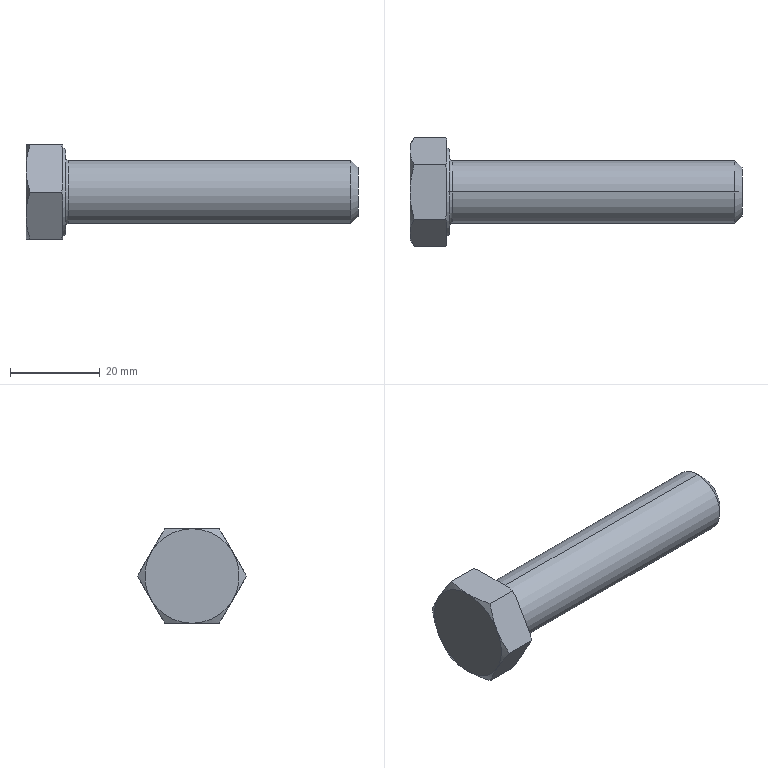Part | SolidWorks | features RevCut 4, Revolution 2, Chamfer 1, Extrusion 1, LPattern 1 | 1 solid | 30 faces | box 73.8 x 24.249 x 21 mm | volume 13256 mm3 | cone 16 | plane 10 | cylinder 2 | torus 2 | commonest cylinder face diameters 14 x2
STEP:
#1=CARTESIAN_POINT('',(9.4,0.,7.));
#2=VERTEX_POINT('',#1);
#3=CARTESIAN_POINT('',(9.4,0.,-7.));
#4=VERTEX_POINT('',#3);
#5=CARTESIAN_POINT('',(9.4,0.,0.));
#6=DIRECTION('',(-1.,0.,0.));
#7=DIRECTION('',(0.,0.,1.));
#8=AXIS2_PLACEMENT_3D('',#5,#6,#7);
#9=CIRCLE('',#8,7.);
#10=EDGE_CURVE('',#2,#4,#9,.T.);
#11=ORIENTED_EDGE('',*,*,#10,.F.);
#12=CARTESIAN_POINT('',(72.2,0.,7.));
#13=VERTEX_POINT('',#12);
#14=CARTESIAN_POINT('',(0.,0.,7.));
#15=DIRECTION('',(1.,0.,0.));
#16=VECTOR('',#15,1000.);
#17=LINE('',#14,#16);
#18=EDGE_CURVE('',#2,#13,#17,.T.);
#19=ORIENTED_EDGE('',*,*,#18,.T.);
#20=CARTESIAN_POINT('',(72.2,0.,-7.));
#21=VERTEX_POINT('',#20);
#22=CARTESIAN_POINT('',(72.2,0.,0.));
#23=DIRECTION('',(-1.,0.,0.));
#24=DIRECTION('',(0.,0.,-1.));
#25=AXIS2_PLACEMENT_3D('',#22,#23,#24);
#26=CIRCLE('',#25,7.);
#27=EDGE_CURVE('',#13,#21,#26,.T.);
#28=ORIENTED_EDGE('',*,*,#27,.T.);
#29=CARTESIAN_POINT('',(0.,0.,-7.));
#30=DIRECTION('',(1.,0.,0.));
#31=VECTOR('',#30,1000.);
#32=LINE('',#29,#31);
#33=EDGE_CURVE('',#4,#21,#32,.T.);
#34=ORIENTED_EDGE('',*,*,#33,.F.);
#35=EDGE_LOOP('',(#11,#19,#28,#34));
#36=FACE_OUTER_BOUND('',#35,.T.);
#37=CARTESIAN_POINT('',(0.,0.,0.));
#38=DIRECTION('',(1.,0.,0.));
#39=DIRECTION('',(0.,0.,-1.));
#40=AXIS2_PLACEMENT_3D('',#37,#38,#39);
#41=CYLINDRICAL_SURFACE('',#40,7.);
#42=ADVANCED_FACE('',(#36),#41,.T.);
#43=CARTESIAN_POINT('',(73.8,0.,-5.4));
#44=VERTEX_POINT('',#43);
#45=CARTESIAN_POINT('',(73.8,0.,5.4));
#46=VERTEX_POINT('',#45);
#47=CARTESIAN_POINT('',(73.8,0.,0.));
#48=DIRECTION('',(1.,0.,0.));
#49=DIRECTION('',(0.,0.,-1.));
#50=AXIS2_PLACEMENT_3D('',#47,#48,#49);
#51=CIRCLE('',#50,5.4);
#52=EDGE_CURVE('',#44,#46,#51,.T.);
#53=ORIENTED_EDGE('',*,*,#52,.F.);
#54=CARTESIAN_POINT('',(73.8,0.,-5.4));
#55=DIRECTION('',(-0.7071,0.,-0.7071));
#56=VECTOR('',#55,1000.);
#57=LINE('',#54,#56);
#58=EDGE_CURVE('',#44,#21,#57,.T.);
#59=ORIENTED_EDGE('',*,*,#58,.T.);
#60=ORIENTED_EDGE('',*,*,#27,.F.);
#61=CARTESIAN_POINT('',(73.8,0.,5.4));
#62=DIRECTION('',(-0.7071,0.,0.7071));
#63=VECTOR('',#62,1000.);
#64=LINE('',#61,#63);
#65=EDGE_CURVE('',#46,#13,#64,.T.);
#66=ORIENTED_EDGE('',*,*,#65,.F.);
#67=EDGE_LOOP('',(#53,#59,#60,#66));
#68=FACE_OUTER_BOUND('',#67,.T.);
#69=CARTESIAN_POINT('',(73.8,0.,0.));
#70=DIRECTION('',(-1.,0.,0.));
#71=DIRECTION('',(0.,0.,1.));
#72=AXIS2_PLACEMENT_3D('',#69,#70,#71);
#73=CONICAL_SURFACE('',#72,5.4,0.7854);
#74=ADVANCED_FACE('',(#68),#73,.T.);
#75=CARTESIAN_POINT('',(8.8,0.,-7.6));
#76=VERTEX_POINT('',#75);
#77=CARTESIAN_POINT('',(8.8,0.,7.6));
#78=VERTEX_POINT('',#77);
#79=CARTESIAN_POINT('',(8.8,0.,0.));
#80=DIRECTION('',(-1.,0.,0.));
#81=DIRECTION('',(0.,0.,1.));
#82=AXIS2_PLACEMENT_3D('',#79,#80,#81);
#83=CIRCLE('',#82,7.6);
#84=EDGE_CURVE('',#76,#78,#83,.T.);
#85=ORIENTED_EDGE('',*,*,#84,.F.);
#86=CARTESIAN_POINT('',(9.4,0.,-7.6));
#87=DIRECTION('',(0.,1.,0.));
#88=DIRECTION('',(0.,0.,1.));
#89=AXIS2_PLACEMENT_3D('',#86,#87,#88);
#90=CIRCLE('',#89,0.6);
#91=EDGE_CURVE('',#76,#4,#90,.T.);
#92=ORIENTED_EDGE('',*,*,#91,.T.);
#93=CARTESIAN_POINT('',(9.4,0.,0.));
#94=DIRECTION('',(-1.,0.,0.));
#95=DIRECTION('',(0.,0.,1.));
#96=AXIS2_PLACEMENT_3D('',#93,#94,#95);
#97=CIRCLE('',#96,7.);
#98=EDGE_CURVE('',#4,#2,#97,.T.);
#99=ORIENTED_EDGE('',*,*,#98,.T.);
#100=CARTESIAN_POINT('',(9.4,0.,7.6));
#101=DIRECTION('',(0.,-1.,0.));
#102=DIRECTION('',(0.,0.,-1.));
#103=AXIS2_PLACEMENT_3D('',#100,#101,#102);
#104=CIRCLE('',#103,0.6);
#105=EDGE_CURVE('',#78,#2,#104,.T.);
#106=ORIENTED_EDGE('',*,*,#105,.F.);
#107=EDGE_LOOP('',(#85,#92,#99,#106));
#108=FACE_OUTER_BOUND('',#107,.T.);
#109=CARTESIAN_POINT('',(9.4,0.,0.));
#110=DIRECTION('',(-1.,0.,0.));
#111=DIRECTION('',(0.,0.,1.));
#112=AXIS2_PLACEMENT_3D('',#109,#110,#111);
#113=TOROIDAL_SURFACE('',#112,7.6,0.6);
#114=ADVANCED_FACE('',(#108),#113,.F.);
#115=CARTESIAN_POINT('',(8.8,0.,9.517));
#116=VERTEX_POINT('',#115);
#117=CARTESIAN_POINT('',(8.8,0.,-9.517));
#118=VERTEX_POINT('',#117);
#119=CARTESIAN_POINT('',(8.8,0.,0.));
#120=DIRECTION('',(-1.,0.,0.));
#121=DIRECTION('',(0.,0.,1.));
#122=AXIS2_PLACEMENT_3D('',#119,#120,#121);
#123=CIRCLE('',#122,9.517);
#124=EDGE_CURVE('',#116,#118,#123,.T.);
#125=ORIENTED_EDGE('',*,*,#124,.T.);
#126=CARTESIAN_POINT('',(8.2,0.,-9.864));
#127=VERTEX_POINT('',#126);
#128=CARTESIAN_POINT('',(8.2,0.,-9.864));
#129=DIRECTION('',(-0.866,0.,-0.5));
#130=VECTOR('',#129,1000.);
#131=LINE('',#128,#130);
#132=EDGE_CURVE('',#118,#127,#131,.T.);
#133=ORIENTED_EDGE('',*,*,#132,.T.);
#134=CARTESIAN_POINT('',(8.2,0.,9.864));
#135=VERTEX_POINT('',#134);
#136=CARTESIAN_POINT('',(8.2,0.,0.));
#137=DIRECTION('',(-1.,0.,0.));
#138=DIRECTION('',(0.,0.,1.));
#139=AXIS2_PLACEMENT_3D('',#136,#137,#138);
#140=CIRCLE('',#139,9.864);
#141=EDGE_CURVE('',#135,#127,#140,.T.);
#142=ORIENTED_EDGE('',*,*,#141,.F.);
#143=CARTESIAN_POINT('',(8.2,0.,9.864));
#144=DIRECTION('',(-0.866,0.,0.5));
#145=VECTOR('',#144,1000.);
#146=LINE('',#143,#145);
#147=EDGE_CURVE('',#116,#135,#146,.T.);
#148=ORIENTED_EDGE('',*,*,#147,.F.);
#149=EDGE_LOOP('',(#125,#133,#142,#148));
#150=FACE_OUTER_BOUND('',#149,.T.);
#151=CARTESIAN_POINT('',(8.2,0.,0.));
#152=DIRECTION('',(-1.,0.,0.));
#153=DIRECTION('',(0.,0.,1.));
#154=AXIS2_PLACEMENT_3D('',#151,#152,#153);
#155=CONICAL_SURFACE('',#154,9.864,0.5236);
#156=ADVANCED_FACE('',(#150),#155,.T.);
#157=ORIENTED_EDGE('',*,*,#124,.F.);
#158=CARTESIAN_POINT('',(8.8,0.,0.));
#159=DIRECTION('',(-1.,0.,0.));
#160=DIRECTION('',(0.,0.,1.));
#161=AXIS2_PLACEMENT_3D('',#158,#159,#160);
#162=CIRCLE('',#161,9.517);
#163=EDGE_CURVE('',#118,#116,#162,.T.);
#164=ORIENTED_EDGE('',*,*,#163,.F.);
#165=EDGE_LOOP('',(#157,#164));
#166=FACE_OUTER_BOUND('',#165,.T.);
#167=CARTESIAN_POINT('',(8.8,0.,0.));
#168=DIRECTION('',(-1.,0.,0.));
#169=DIRECTION('',(0.,0.,1.));
#170=AXIS2_PLACEMENT_3D('',#167,#168,#169);
#171=CIRCLE('',#170,7.6);
#172=EDGE_CURVE('',#78,#76,#171,.T.);
#173=ORIENTED_EDGE('',*,*,#172,.T.);
#174=ORIENTED_EDGE('',*,*,#84,.T.);
#175=EDGE_LOOP('',(#173,#174));
#176=FACE_BOUND('',#175,.T.);
#177=CARTESIAN_POINT('',(8.8,12.124,0.));
#178=DIRECTION('',(1.,0.,0.));
#179=DIRECTION('',(0.,0.,-1.));
#180=AXIS2_PLACEMENT_3D('',#177,#178,#179);
#181=PLANE('',#180);
#182=ADVANCED_FACE('',(#166,#176),#181,.T.);
#183=CARTESIAN_POINT('',(8.2,6.7,-9.395));
#184=VERTEX_POINT('',#183);
#185=CARTESIAN_POINT('',(8.2,11.486,-1.105));
#186=VERTEX_POINT('',#185);
#187=CARTESIAN_POINT('',(8.2,6.062,-10.5));
#188=DIRECTION('',(0.,0.5,0.866));
#189=VECTOR('',#188,1000.);
#190=LINE('',#187,#189);
#191=EDGE_CURVE('',#184,#186,#190,.T.);
#192=ORIENTED_EDGE('',*,*,#191,.F.);
#193=CARTESIAN_POINT('',(7.862,6.062,-10.5));
#194=VERTEX_POINT('',#193);
#195=CARTESIAN_POINT('',(7.862,6.062,-10.5));
#196=CARTESIAN_POINT('',(7.985,6.274,-10.133));
#197=CARTESIAN_POINT('',(8.098,6.487,-9.764));
#198=CARTESIAN_POINT('',(8.2,6.7,-9.395));
#199=B_SPLINE_CURVE_WITH_KNOTS('',3,(#195,#196,#197,#198),.UNSPECIFIED.,.F.,.F.,(4,4),(0.000000238,0.001312),.UNSPECIFIED.);
#200=EDGE_CURVE('',#194,#184,#199,.T.);
#201=ORIENTED_EDGE('',*,*,#200,.F.);
#202=CARTESIAN_POINT('',(0.9378,6.062,-10.5));
#203=VERTEX_POINT('',#202);
#204=CARTESIAN_POINT('',(8.8,6.062,-10.5));
#205=DIRECTION('',(-1.,0.,0.));
#206=VECTOR('',#205,1000.);
#207=LINE('',#204,#206);
#208=EDGE_CURVE('',#194,#203,#207,.T.);
#209=ORIENTED_EDGE('',*,*,#208,.T.);
#210=CARTESIAN_POINT('',(0.,9.093,-5.25));
#211=VERTEX_POINT('',#210);
#212=CARTESIAN_POINT('',(0.,9.093,-5.25));
#213=CARTESIAN_POINT('',(0.,8.836,-5.696));
#214=CARTESIAN_POINT('',(0.02217,8.578,-6.143));
#215=CARTESIAN_POINT('',(0.1079,8.066,-7.028));
#216=CARTESIAN_POINT('',(0.1715,7.813,-7.468));
#217=CARTESIAN_POINT('',(0.4165,7.056,-8.779));
#218=CARTESIAN_POINT('',(0.6523,6.557,-9.643));
#219=CARTESIAN_POINT('',(0.9378,6.062,-10.5));
#220=B_SPLINE_CURVE_WITH_KNOTS('',3,(#212,#213,#214,#215,#216,#217,#218,#219),.UNSPECIFIED.,.F.,.F.,(4,2,2,4),(0.006134,0.007662,0.00919,0.01225),.UNSPECIFIED.);
#221=EDGE_CURVE('',#211,#203,#220,.T.);
#222=ORIENTED_EDGE('',*,*,#221,.F.);
#223=CARTESIAN_POINT('',(0.9378,12.124,0.));
#224=VERTEX_POINT('',#223);
#225=CARTESIAN_POINT('',(0.9378,12.124,0.));
#226=CARTESIAN_POINT('',(0.6515,11.629,-0.8588));
#227=CARTESIAN_POINT('',(0.4157,11.129,-1.724));
#228=CARTESIAN_POINT('',(0.08938,10.12,-3.472));
#229=CARTESIAN_POINT('',(0.,9.61,-4.356));
#230=CARTESIAN_POINT('',(0.,9.093,-5.25));
#231=B_SPLINE_CURVE_WITH_KNOTS('',3,(#225,#226,#227,#228,#229,#230),.UNSPECIFIED.,.F.,.F.,(4,2,4),(0.000000238,0.003067,0.006134),.UNSPECIFIED.);
#232=EDGE_CURVE('',#224,#211,#231,.T.);
#233=ORIENTED_EDGE('',*,*,#232,.F.);
#234=CARTESIAN_POINT('',(7.862,12.124,0.));
#235=VERTEX_POINT('',#234);
#236=CARTESIAN_POINT('',(8.8,12.124,0.));
#237=DIRECTION('',(-1.,0.,0.));
#238=VECTOR('',#237,1000.);
#239=LINE('',#236,#238);
#240=EDGE_CURVE('',#235,#224,#239,.T.);
#241=ORIENTED_EDGE('',*,*,#240,.F.);
#242=CARTESIAN_POINT('',(8.2,11.486,-1.105));
#243=CARTESIAN_POINT('',(8.098,11.7,-0.7354));
#244=CARTESIAN_POINT('',(7.985,11.912,-0.3671));
#245=CARTESIAN_POINT('',(7.862,12.124,0.));
#246=B_SPLINE_CURVE_WITH_KNOTS('',3,(#242,#243,#244,#245),.UNSPECIFIED.,.F.,.F.,(4,4),(0.01094,0.01225),.UNSPECIFIED.);
#247=EDGE_CURVE('',#186,#235,#246,.T.);
#248=ORIENTED_EDGE('',*,*,#247,.F.);
#249=EDGE_LOOP('',(#192,#201,#209,#222,#233,#241,#248));
#250=FACE_OUTER_BOUND('',#249,.T.);
#251=CARTESIAN_POINT('',(8.8,6.062,-10.5));
#252=DIRECTION('',(0.,-0.866,0.5));
#253=DIRECTION('',(0.,-0.5,-0.866));
#254=AXIS2_PLACEMENT_3D('',#251,#252,#253);
#255=PLANE('',#254);
#256=ADVANCED_FACE('',(#250),#255,.F.);
#257=CARTESIAN_POINT('',(8.2,11.486,1.105));
#258=VERTEX_POINT('',#257);
#259=CARTESIAN_POINT('',(8.2,6.7,9.395));
#260=VERTEX_POINT('',#259);
#261=CARTESIAN_POINT('',(8.2,12.124,0.));
#262=DIRECTION('',(0.,-0.5,0.866));
#263=VECTOR('',#262,1000.);
#264=LINE('',#261,#263);
#265=EDGE_CURVE('',#258,#260,#264,.T.);
#266=ORIENTED_EDGE('',*,*,#265,.F.);
#267=CARTESIAN_POINT('',(7.862,12.124,0.));
#268=CARTESIAN_POINT('',(7.985,11.912,0.3672));
#269=CARTESIAN_POINT('',(8.098,11.7,0.7356));
#270=CARTESIAN_POINT('',(8.2,11.486,1.105));
#271=B_SPLINE_CURVE_WITH_KNOTS('',3,(#267,#268,#269,#270),.UNSPECIFIED.,.F.,.F.,(4,4),(0.000000238,0.001312),.UNSPECIFIED.);
#272=EDGE_CURVE('',#235,#258,#271,.T.);
#273=ORIENTED_EDGE('',*,*,#272,.F.);
#274=ORIENTED_EDGE('',*,*,#240,.T.);
#275=CARTESIAN_POINT('',(0.,9.093,5.25));
#276=VERTEX_POINT('',#275);
#277=CARTESIAN_POINT('',(0.,9.093,5.25));
#278=CARTESIAN_POINT('',(0.,9.351,4.804));
#279=CARTESIAN_POINT('',(0.02217,9.609,4.357));
#280=CARTESIAN_POINT('',(0.1079,10.12,3.472));
#281=CARTESIAN_POINT('',(0.1715,10.374,3.032));
#282=CARTESIAN_POINT('',(0.4165,11.131,1.721));
#283=CARTESIAN_POINT('',(0.6523,11.63,0.8567));
#284=CARTESIAN_POINT('',(0.9378,12.124,0.));
#285=B_SPLINE_CURVE_WITH_KNOTS('',3,(#277,#278,#279,#280,#281,#282,#283,#284),.UNSPECIFIED.,.F.,.F.,(4,2,2,4),(0.006134,0.007662,0.00919,0.01225),.UNSPECIFIED.);
#286=EDGE_CURVE('',#276,#224,#285,.T.);
#287=ORIENTED_EDGE('',*,*,#286,.F.);
#288=CARTESIAN_POINT('',(0.9378,6.062,10.5));
#289=VERTEX_POINT('',#288);
#290=CARTESIAN_POINT('',(0.9378,6.062,10.5));
#291=CARTESIAN_POINT('',(0.6515,6.558,9.641));
#292=CARTESIAN_POINT('',(0.4157,7.057,8.776));
#293=CARTESIAN_POINT('',(0.08938,8.067,7.028));
#294=CARTESIAN_POINT('',(0.,8.577,6.144));
#295=CARTESIAN_POINT('',(0.,9.093,5.25));
#296=B_SPLINE_CURVE_WITH_KNOTS('',3,(#290,#291,#292,#293,#294,#295),.UNSPECIFIED.,.F.,.F.,(4,2,4),(0.000000238,0.003067,0.006134),.UNSPECIFIED.);
#297=EDGE_CURVE('',#289,#276,#296,.T.);
#298=ORIENTED_EDGE('',*,*,#297,.F.);
#299=CARTESIAN_POINT('',(7.862,6.062,10.5));
#300=VERTEX_POINT('',#299);
#301=CARTESIAN_POINT('',(8.8,6.062,10.5));
#302=DIRECTION('',(-1.,0.,0.));
#303=VECTOR('',#302,1000.);
#304=LINE('',#301,#303);
#305=EDGE_CURVE('',#300,#289,#304,.T.);
#306=ORIENTED_EDGE('',*,*,#305,.F.);
#307=CARTESIAN_POINT('',(8.2,6.7,9.395));
#308=CARTESIAN_POINT('',(8.098,6.487,9.765));
#309=CARTESIAN_POINT('',(7.985,6.274,10.133));
#310=CARTESIAN_POINT('',(7.862,6.062,10.5));
#311=B_SPLINE_CURVE_WITH_KNOTS('',3,(#307,#308,#309,#310),.UNSPECIFIED.,.F.,.F.,(4,4),(0.01094,0.01225),.UNSPECIFIED.);
#312=EDGE_CURVE('',#260,#300,#311,.T.);
#313=ORIENTED_EDGE('',*,*,#312,.F.);
#314=EDGE_LOOP('',(#266,#273,#274,#287,#298,#306,#313));
#315=FACE_OUTER_BOUND('',#314,.T.);
#316=CARTESIAN_POINT('',(8.8,12.124,0.));
#317=DIRECTION('',(0.,-0.866,-0.5));
#318=DIRECTION('',(0.,0.5,-0.866));
#319=AXIS2_PLACEMENT_3D('',#316,#317,#318);
#320=PLANE('',#319);
#321=ADVANCED_FACE('',(#315),#320,.F.);
#322=CARTESIAN_POINT('',(8.2,4.786,10.5));
#323=VERTEX_POINT('',#322);
#324=CARTESIAN_POINT('',(8.2,-4.786,10.5));
#325=VERTEX_POINT('',#324);
#326=CARTESIAN_POINT('',(8.2,6.062,10.5));
#327=DIRECTION('',(0.,-1.,0.));
#328=VECTOR('',#327,1000.);
#329=LINE('',#326,#328);
#330=EDGE_CURVE('',#323,#325,#329,.T.);
#331=ORIENTED_EDGE('',*,*,#330,.F.);
#332=CARTESIAN_POINT('',(7.862,6.062,10.5));
#333=CARTESIAN_POINT('',(7.984,5.639,10.5));
#334=CARTESIAN_POINT('',(8.097,5.214,10.5));
#335=CARTESIAN_POINT('',(8.2,4.786,10.5));
#336=B_SPLINE_CURVE_WITH_KNOTS('',3,(#332,#333,#334,#335),.UNSPECIFIED.,.F.,.F.,(4,4),(0.02875,0.03008),.UNSPECIFIED.);
#337=EDGE_CURVE('',#300,#323,#336,.T.);
#338=ORIENTED_EDGE('',*,*,#337,.F.);
#339=ORIENTED_EDGE('',*,*,#305,.T.);
#340=CARTESIAN_POINT('',(0.,0.,10.5));
#341=VERTEX_POINT('',#340);
#342=CARTESIAN_POINT('',(0.,0.,10.5));
#343=CARTESIAN_POINT('',(0.,0.5133,10.5));
#344=CARTESIAN_POINT('',(0.02195,1.03,10.5));
#345=CARTESIAN_POINT('',(0.1087,2.061,10.5));
#346=CARTESIAN_POINT('',(0.1729,2.572,10.5));
#347=CARTESIAN_POINT('',(0.4192,4.089,10.5));
#348=CARTESIAN_POINT('',(0.6548,5.082,10.5));
#349=CARTESIAN_POINT('',(0.9378,6.062,10.5));
#350=B_SPLINE_CURVE_WITH_KNOTS('',3,(#342,#343,#344,#345,#346,#347,#348,#349),.UNSPECIFIED.,.F.,.F.,(4,2,2,4),(0.0174,0.01894,0.02047,0.02354),.UNSPECIFIED.);
#351=EDGE_CURVE('',#341,#289,#350,.T.);
#352=ORIENTED_EDGE('',*,*,#351,.F.);
#353=CARTESIAN_POINT('',(0.9378,-6.062,10.5));
#354=VERTEX_POINT('',#353);
#355=CARTESIAN_POINT('',(0.9378,-6.062,10.5));
#356=CARTESIAN_POINT('',(0.6528,-5.075,10.5));
#357=CARTESIAN_POINT('',(0.4144,-4.066,10.5));
#358=CARTESIAN_POINT('',(0.08826,-2.044,10.5));
#359=CARTESIAN_POINT('',(0.,-1.026,10.5));
#360=CARTESIAN_POINT('',(0.,0.,10.5));
#361=B_SPLINE_CURVE_WITH_KNOTS('',3,(#355,#356,#357,#358,#359,#360),.UNSPECIFIED.,.F.,.F.,(4,2,4),(0.01126,0.01433,0.0174),.UNSPECIFIED.);
#362=EDGE_CURVE('',#354,#341,#361,.T.);
#363=ORIENTED_EDGE('',*,*,#362,.F.);
#364=CARTESIAN_POINT('',(7.862,-6.062,10.5));
#365=VERTEX_POINT('',#364);
#366=CARTESIAN_POINT('',(8.8,-6.062,10.5));
#367=DIRECTION('',(-1.,0.,0.));
#368=VECTOR('',#367,1000.);
#369=LINE('',#366,#368);
#370=EDGE_CURVE('',#365,#354,#369,.T.);
#371=ORIENTED_EDGE('',*,*,#370,.F.);
#372=CARTESIAN_POINT('',(8.2,-4.786,10.5));
#373=CARTESIAN_POINT('',(8.097,-5.215,10.5));
#374=CARTESIAN_POINT('',(7.984,-5.64,10.5));
#375=CARTESIAN_POINT('',(7.862,-6.062,10.5));
#376=B_SPLINE_CURVE_WITH_KNOTS('',3,(#372,#373,#374,#375),.UNSPECIFIED.,.F.,.F.,(4,4),(0.03972,0.04103),.UNSPECIFIED.);
#377=EDGE_CURVE('',#325,#365,#376,.T.);
#378=ORIENTED_EDGE('',*,*,#377,.F.);
#379=EDGE_LOOP('',(#331,#338,#339,#352,#363,#371,#378));
#380=FACE_OUTER_BOUND('',#379,.T.);
#381=CARTESIAN_POINT('',(8.8,6.062,10.5));
#382=DIRECTION('',(0.,0.,-1.));
#383=DIRECTION('',(0.,1.,0.));
#384=AXIS2_PLACEMENT_3D('',#381,#382,#383);
#385=PLANE('',#384);
#386=ADVANCED_FACE('',(#380),#385,.F.);
#387=CARTESIAN_POINT('',(8.2,-6.7,9.395));
#388=VERTEX_POINT('',#387);
#389=CARTESIAN_POINT('',(8.2,-11.486,1.105));
#390=VERTEX_POINT('',#389);
#391=CARTESIAN_POINT('',(8.2,-12.124,0.));
#392=DIRECTION('',(0.,-0.5,-0.866));
#393=VECTOR('',#392,1000.);
#394=LINE('',#391,#393);
#395=EDGE_CURVE('',#388,#390,#394,.T.);
#396=ORIENTED_EDGE('',*,*,#395,.F.);
#397=CARTESIAN_POINT('',(7.862,-6.062,10.5));
#398=CARTESIAN_POINT('',(7.985,-6.274,10.133));
#399=CARTESIAN_POINT('',(8.098,-6.487,9.764));
#400=CARTESIAN_POINT('',(8.2,-6.7,9.395));
#401=B_SPLINE_CURVE_WITH_KNOTS('',3,(#397,#398,#399,#400),.UNSPECIFIED.,.F.,.F.,(4,4),(0.000000238,0.001312),.UNSPECIFIED.);
#402=EDGE_CURVE('',#365,#388,#401,.T.);
#403=ORIENTED_EDGE('',*,*,#402,.F.);
#404=ORIENTED_EDGE('',*,*,#370,.T.);
#405=CARTESIAN_POINT('',(0.,-9.093,5.25));
#406=VERTEX_POINT('',#405);
#407=CARTESIAN_POINT('',(0.,-9.093,5.25));
#408=CARTESIAN_POINT('',(0.,-8.836,5.696));
#409=CARTESIAN_POINT('',(0.02217,-8.578,6.143));
#410=CARTESIAN_POINT('',(0.1079,-8.066,7.028));
#411=CARTESIAN_POINT('',(0.1715,-7.813,7.468));
#412=CARTESIAN_POINT('',(0.4165,-7.056,8.779));
#413=CARTESIAN_POINT('',(0.6523,-6.557,9.643));
#414=CARTESIAN_POINT('',(0.9378,-6.062,10.5));
#415=B_SPLINE_CURVE_WITH_KNOTS('',3,(#407,#408,#409,#410,#411,#412,#413,#414),.UNSPECIFIED.,.F.,.F.,(4,2,2,4),(0.006134,0.007662,0.00919,0.01225),.UNSPECIFIED.);
#416=EDGE_CURVE('',#406,#354,#415,.T.);
#417=ORIENTED_EDGE('',*,*,#416,.F.);
#418=CARTESIAN_POINT('',(0.9378,-12.124,0.));
#419=VERTEX_POINT('',#418);
#420=CARTESIAN_POINT('',(0.9378,-12.124,0.));
#421=CARTESIAN_POINT('',(0.6515,-11.629,0.8588));
#422=CARTESIAN_POINT('',(0.4157,-11.129,1.724));
#423=CARTESIAN_POINT('',(0.08938,-10.12,3.472));
#424=CARTESIAN_POINT('',(0.,-9.61,4.356));
#425=CARTESIAN_POINT('',(0.,-9.093,5.25));
#426=B_SPLINE_CURVE_WITH_KNOTS('',3,(#420,#421,#422,#423,#424,#425),.UNSPECIFIED.,.F.,.F.,(4,2,4),(0.000000238,0.003067,0.006134),.UNSPECIFIED.);
#427=EDGE_CURVE('',#419,#406,#426,.T.);
#428=ORIENTED_EDGE('',*,*,#427,.F.);
#429=CARTESIAN_POINT('',(7.862,-12.124,0.));
#430=VERTEX_POINT('',#429);
#431=CARTESIAN_POINT('',(8.8,-12.124,0.));
#432=DIRECTION('',(-1.,0.,0.));
#433=VECTOR('',#432,1000.);
#434=LINE('',#431,#433);
#435=EDGE_CURVE('',#430,#419,#434,.T.);
#436=ORIENTED_EDGE('',*,*,#435,.F.);
#437=CARTESIAN_POINT('',(8.2,-11.486,1.105));
#438=CARTESIAN_POINT('',(8.098,-11.7,0.7354));
#439=CARTESIAN_POINT('',(7.985,-11.912,0.3671));
#440=CARTESIAN_POINT('',(7.862,-12.124,0.));
#441=B_SPLINE_CURVE_WITH_KNOTS('',3,(#437,#438,#439,#440),.UNSPECIFIED.,.F.,.F.,(4,4),(0.01094,0.01225),.UNSPECIFIED.);
#442=EDGE_CURVE('',#390,#430,#441,.T.);
#443=ORIENTED_EDGE('',*,*,#442,.F.);
#444=EDGE_LOOP('',(#396,#403,#404,#417,#428,#436,#443));
#445=FACE_OUTER_BOUND('',#444,.T.);
#446=CARTESIAN_POINT('',(8.8,-12.124,0.));
#447=DIRECTION('',(0.,0.866,-0.5));
#448=DIRECTION('',(0.,0.5,0.866));
#449=AXIS2_PLACEMENT_3D('',#446,#447,#448);
#450=PLANE('',#449);
#451=ADVANCED_FACE('',(#445),#450,.F.);
#452=CARTESIAN_POINT('',(8.2,-11.486,-1.105));
#453=VERTEX_POINT('',#452);
#454=CARTESIAN_POINT('',(8.2,-6.7,-9.395));
#455=VERTEX_POINT('',#454);
#456=CARTESIAN_POINT('',(8.2,-6.062,-10.5));
#457=DIRECTION('',(0.,0.5,-0.866));
#458=VECTOR('',#457,1000.);
#459=LINE('',#456,#458);
#460=EDGE_CURVE('',#453,#455,#459,.T.);
#461=ORIENTED_EDGE('',*,*,#460,.F.);
#462=CARTESIAN_POINT('',(7.862,-12.124,0.));
#463=CARTESIAN_POINT('',(7.985,-11.912,-0.3672));
#464=CARTESIAN_POINT('',(8.098,-11.7,-0.7356));
#465=CARTESIAN_POINT('',(8.2,-11.486,-1.105));
#466=B_SPLINE_CURVE_WITH_KNOTS('',3,(#462,#463,#464,#465),.UNSPECIFIED.,.F.,.F.,(4,4),(0.000000238,0.001312),.UNSPECIFIED.);
#467=EDGE_CURVE('',#430,#453,#466,.T.);
#468=ORIENTED_EDGE('',*,*,#467,.F.);
#469=ORIENTED_EDGE('',*,*,#435,.T.);
#470=CARTESIAN_POINT('',(0.,-9.093,-5.25));
#471=VERTEX_POINT('',#470);
#472=CARTESIAN_POINT('',(0.,-9.093,-5.25));
#473=CARTESIAN_POINT('',(0.,-9.351,-4.804));
#474=CARTESIAN_POINT('',(0.02217,-9.609,-4.357));
#475=CARTESIAN_POINT('',(0.1079,-10.12,-3.472));
#476=CARTESIAN_POINT('',(0.1715,-10.374,-3.032));
#477=CARTESIAN_POINT('',(0.4165,-11.131,-1.721));
#478=CARTESIAN_POINT('',(0.6523,-11.63,-0.8567));
#479=CARTESIAN_POINT('',(0.9378,-12.124,0.));
#480=B_SPLINE_CURVE_WITH_KNOTS('',3,(#472,#473,#474,#475,#476,#477,#478,#479),.UNSPECIFIED.,.F.,.F.,(4,2,2,4),(0.006134,0.007662,0.00919,0.01225),.UNSPECIFIED.);
#481=EDGE_CURVE('',#471,#419,#480,.T.);
#482=ORIENTED_EDGE('',*,*,#481,.F.);
#483=CARTESIAN_POINT('',(0.9378,-6.062,-10.5));
#484=VERTEX_POINT('',#483);
#485=CARTESIAN_POINT('',(0.9378,-6.062,-10.5));
#486=CARTESIAN_POINT('',(0.6515,-6.558,-9.641));
#487=CARTESIAN_POINT('',(0.4157,-7.057,-8.776));
#488=CARTESIAN_POINT('',(0.08938,-8.067,-7.028));
#489=CARTESIAN_POINT('',(0.,-8.577,-6.144));
#490=CARTESIAN_POINT('',(0.,-9.093,-5.25));
#491=B_SPLINE_CURVE_WITH_KNOTS('',3,(#485,#486,#487,#488,#489,#490),.UNSPECIFIED.,.F.,.F.,(4,2,4),(0.000000238,0.003067,0.006134),.UNSPECIFIED.);
#492=EDGE_CURVE('',#484,#471,#491,.T.);
#493=ORIENTED_EDGE('',*,*,#492,.F.);
#494=CARTESIAN_POINT('',(7.862,-6.062,-10.5));
#495=VERTEX_POINT('',#494);
#496=CARTESIAN_POINT('',(8.8,-6.062,-10.5));
#497=DIRECTION('',(-1.,0.,0.));
#498=VECTOR('',#497,1000.);
#499=LINE('',#496,#498);
#500=EDGE_CURVE('',#495,#484,#499,.T.);
#501=ORIENTED_EDGE('',*,*,#500,.F.);
#502=CARTESIAN_POINT('',(8.2,-6.7,-9.395));
#503=CARTESIAN_POINT('',(8.098,-6.487,-9.765));
#504=CARTESIAN_POINT('',(7.985,-6.274,-10.133));
#505=CARTESIAN_POINT('',(7.862,-6.062,-10.5));
#506=B_SPLINE_CURVE_WITH_KNOTS('',3,(#502,#503,#504,#505),.UNSPECIFIED.,.F.,.F.,(4,4),(0.01094,0.01225),.UNSPECIFIED.);
#507=EDGE_CURVE('',#455,#495,#506,.T.);
#508=ORIENTED_EDGE('',*,*,#507,.F.);
#509=EDGE_LOOP('',(#461,#468,#469,#482,#493,#501,#508));
#510=FACE_OUTER_BOUND('',#509,.T.);
#511=CARTESIAN_POINT('',(8.8,-6.062,-10.5));
#512=DIRECTION('',(0.,0.866,0.5));
#513=DIRECTION('',(0.,-0.5,0.866));
#514=AXIS2_PLACEMENT_3D('',#511,#512,#513);
#515=PLANE('',#514);
#516=ADVANCED_FACE('',(#510),#515,.F.);
#517=CARTESIAN_POINT('',(8.2,-4.786,-10.5));
#518=VERTEX_POINT('',#517);
#519=CARTESIAN_POINT('',(8.2,4.786,-10.5));
#520=VERTEX_POINT('',#519);
#521=CARTESIAN_POINT('',(8.2,6.062,-10.5));
#522=DIRECTION('',(0.,1.,0.));
#523=VECTOR('',#522,1000.);
#524=LINE('',#521,#523);
#525=EDGE_CURVE('',#518,#520,#524,.T.);
#526=ORIENTED_EDGE('',*,*,#525,.F.);
#527=CARTESIAN_POINT('',(7.862,-6.062,-10.5));
#528=CARTESIAN_POINT('',(7.984,-5.64,-10.5));
#529=CARTESIAN_POINT('',(8.097,-5.215,-10.5));
#530=CARTESIAN_POINT('',(8.2,-4.786,-10.5));
#531=B_SPLINE_CURVE_WITH_KNOTS('',3,(#527,#528,#529,#530),.UNSPECIFIED.,.F.,.F.,(4,4),(0.01126,0.01258),.UNSPECIFIED.);
#532=EDGE_CURVE('',#495,#518,#531,.T.);
#533=ORIENTED_EDGE('',*,*,#532,.F.);
#534=ORIENTED_EDGE('',*,*,#500,.T.);
#535=CARTESIAN_POINT('',(0.,0.,-10.5));
#536=VERTEX_POINT('',#535);
#537=CARTESIAN_POINT('',(0.,0.,-10.5));
#538=CARTESIAN_POINT('',(0.,-1.026,-10.5));
#539=CARTESIAN_POINT('',(0.08826,-2.044,-10.5));
#540=CARTESIAN_POINT('',(0.4144,-4.066,-10.5));
#541=CARTESIAN_POINT('',(0.6528,-5.075,-10.5));
#542=CARTESIAN_POINT('',(0.9378,-6.062,-10.5));
#543=B_SPLINE_CURVE_WITH_KNOTS('',3,(#537,#538,#539,#540,#541,#542),.UNSPECIFIED.,.F.,.F.,(4,2,4),(0.03489,0.03796,0.04103),.UNSPECIFIED.);
#544=EDGE_CURVE('',#536,#484,#543,.T.);
#545=ORIENTED_EDGE('',*,*,#544,.F.);
#546=CARTESIAN_POINT('',(0.9378,6.062,-10.5));
#547=CARTESIAN_POINT('',(0.6548,5.082,-10.5));
#548=CARTESIAN_POINT('',(0.4192,4.089,-10.5));
#549=CARTESIAN_POINT('',(0.1729,2.572,-10.5));
#550=CARTESIAN_POINT('',(0.1087,2.061,-10.5));
#551=CARTESIAN_POINT('',(0.02195,1.03,-10.5));
#552=CARTESIAN_POINT('',(0.,0.5133,-10.5));
#553=CARTESIAN_POINT('',(0.,0.,-10.5));
#554=B_SPLINE_CURVE_WITH_KNOTS('',3,(#546,#547,#548,#549,#550,#551,#552,#553),.UNSPECIFIED.,.F.,.F.,(4,2,2,4),(0.02875,0.03182,0.03336,0.03489),.UNSPECIFIED.);
#555=EDGE_CURVE('',#203,#536,#554,.T.);
#556=ORIENTED_EDGE('',*,*,#555,.F.);
#557=ORIENTED_EDGE('',*,*,#208,.F.);
#558=CARTESIAN_POINT('',(8.2,4.786,-10.5));
#559=CARTESIAN_POINT('',(8.097,5.214,-10.5));
#560=CARTESIAN_POINT('',(7.984,5.639,-10.5));
#561=CARTESIAN_POINT('',(7.862,6.062,-10.5));
#562=B_SPLINE_CURVE_WITH_KNOTS('',3,(#558,#559,#560,#561),.UNSPECIFIED.,.F.,.F.,(4,4),(0.02222,0.02354),.UNSPECIFIED.);
#563=EDGE_CURVE('',#520,#194,#562,.T.);
#564=ORIENTED_EDGE('',*,*,#563,.F.);
#565=EDGE_LOOP('',(#526,#533,#534,#545,#556,#557,#564));
#566=FACE_OUTER_BOUND('',#565,.T.);
#567=CARTESIAN_POINT('',(8.8,6.062,-10.5));
#568=DIRECTION('',(0.,0.,1.));
#569=DIRECTION('',(1.,0.,0.));
#570=AXIS2_PLACEMENT_3D('',#567,#568,#569);
#571=PLANE('',#570);
#572=ADVANCED_FACE('',(#566),#571,.F.);
#573=ORIENTED_EDGE('',*,*,#532,.T.);
#574=CARTESIAN_POINT('',(8.2,0.,0.));
#575=DIRECTION('',(-1.,0.,0.));
#576=DIRECTION('',(0.,0.,-1.));
#577=AXIS2_PLACEMENT_3D('',#574,#575,#576);
#578=CIRCLE('',#577,11.539);
#579=EDGE_CURVE('',#518,#455,#578,.T.);
#580=ORIENTED_EDGE('',*,*,#579,.T.);
#581=ORIENTED_EDGE('',*,*,#507,.T.);
#582=EDGE_LOOP('',(#573,#580,#581));
#583=FACE_OUTER_BOUND('',#582,.T.);
#584=CARTESIAN_POINT('',(4.975,0.,0.));
#585=DIRECTION('',(-1.,0.,0.));
#586=DIRECTION('',(0.,0.,1.));
#587=AXIS2_PLACEMENT_3D('',#584,#585,#586);
#588=CONICAL_SURFACE('',#587,17.124,1.047);
#589=ADVANCED_FACE('',(#583),#588,.T.);
#590=ORIENTED_EDGE('',*,*,#467,.T.);
#591=CARTESIAN_POINT('',(8.2,0.,0.));
#592=DIRECTION('',(-1.,0.,0.));
#593=DIRECTION('',(0.,0.,-1.));
#594=AXIS2_PLACEMENT_3D('',#591,#592,#593);
#595=CIRCLE('',#594,11.539);
#596=EDGE_CURVE('',#453,#390,#595,.T.);
#597=ORIENTED_EDGE('',*,*,#596,.T.);
#598=ORIENTED_EDGE('',*,*,#442,.T.);
#599=EDGE_LOOP('',(#590,#597,#598));
#600=FACE_OUTER_BOUND('',#599,.T.);
#601=CARTESIAN_POINT('',(4.975,0.,0.));
#602=DIRECTION('',(-1.,0.,0.));
#603=DIRECTION('',(0.,0.,1.));
#604=AXIS2_PLACEMENT_3D('',#601,#602,#603);
#605=CONICAL_SURFACE('',#604,17.124,1.047);
#606=ADVANCED_FACE('',(#600),#605,.T.);
#607=ORIENTED_EDGE('',*,*,#402,.T.);
#608=CARTESIAN_POINT('',(8.2,0.,0.));
#609=DIRECTION('',(-1.,0.,0.));
#610=DIRECTION('',(0.,0.,-1.));
#611=AXIS2_PLACEMENT_3D('',#608,#609,#610);
#612=CIRCLE('',#611,11.539);
#613=EDGE_CURVE('',#388,#325,#612,.T.);
#614=ORIENTED_EDGE('',*,*,#613,.T.);
#615=ORIENTED_EDGE('',*,*,#377,.T.);
#616=EDGE_LOOP('',(#607,#614,#615));
#617=FACE_OUTER_BOUND('',#616,.T.);
#618=CARTESIAN_POINT('',(4.975,0.,0.));
#619=DIRECTION('',(-1.,0.,0.));
#620=DIRECTION('',(0.,0.,1.));
#621=AXIS2_PLACEMENT_3D('',#618,#619,#620);
#622=CONICAL_SURFACE('',#621,17.124,1.047);
#623=ADVANCED_FACE('',(#617),#622,.T.);
#624=ORIENTED_EDGE('',*,*,#337,.T.);
#625=CARTESIAN_POINT('',(8.2,0.,0.));
#626=DIRECTION('',(-1.,0.,0.));
#627=DIRECTION('',(0.,0.,-1.));
#628=AXIS2_PLACEMENT_3D('',#625,#626,#627);
#629=CIRCLE('',#628,11.539);
#630=EDGE_CURVE('',#323,#260,#629,.T.);
#631=ORIENTED_EDGE('',*,*,#630,.T.);
#632=ORIENTED_EDGE('',*,*,#312,.T.);
#633=EDGE_LOOP('',(#624,#631,#632));
#634=FACE_OUTER_BOUND('',#633,.T.);
#635=CARTESIAN_POINT('',(4.975,0.,0.));
#636=DIRECTION('',(-1.,0.,0.));
#637=DIRECTION('',(0.,0.,1.));
#638=AXIS2_PLACEMENT_3D('',#635,#636,#637);
#639=CONICAL_SURFACE('',#638,17.124,1.047);
#640=ADVANCED_FACE('',(#634),#639,.T.);
#641=ORIENTED_EDGE('',*,*,#272,.T.);
#642=CARTESIAN_POINT('',(8.2,0.,0.));
#643=DIRECTION('',(-1.,0.,0.));
#644=DIRECTION('',(0.,0.,-1.));
#645=AXIS2_PLACEMENT_3D('',#642,#643,#644);
#646=CIRCLE('',#645,11.539);
#647=EDGE_CURVE('',#258,#186,#646,.T.);
#648=ORIENTED_EDGE('',*,*,#647,.T.);
#649=ORIENTED_EDGE('',*,*,#247,.T.);
#650=EDGE_LOOP('',(#641,#648,#649));
#651=FACE_OUTER_BOUND('',#650,.T.);
#652=CARTESIAN_POINT('',(4.975,0.,0.));
#653=DIRECTION('',(-1.,0.,0.));
#654=DIRECTION('',(0.,0.,1.));
#655=AXIS2_PLACEMENT_3D('',#652,#653,#654);
#656=CONICAL_SURFACE('',#655,17.124,1.047);
#657=ADVANCED_FACE('',(#651),#656,.T.);
#658=ORIENTED_EDGE('',*,*,#200,.T.);
#659=CARTESIAN_POINT('',(8.2,0.,0.));
#660=DIRECTION('',(-1.,0.,0.));
#661=DIRECTION('',(0.,0.,-1.));
#662=AXIS2_PLACEMENT_3D('',#659,#660,#661);
#663=CIRCLE('',#662,11.539);
#664=EDGE_CURVE('',#184,#520,#663,.T.);
#665=ORIENTED_EDGE('',*,*,#664,.T.);
#666=ORIENTED_EDGE('',*,*,#563,.T.);
#667=EDGE_LOOP('',(#658,#665,#666));
#668=FACE_OUTER_BOUND('',#667,.T.);
#669=CARTESIAN_POINT('',(4.975,0.,0.));
#670=DIRECTION('',(-1.,0.,0.));
#671=DIRECTION('',(0.,0.,1.));
#672=AXIS2_PLACEMENT_3D('',#669,#670,#671);
#673=CONICAL_SURFACE('',#672,17.124,1.047);
#674=ADVANCED_FACE('',(#668),#673,.T.);
#675=ORIENTED_EDGE('',*,*,#492,.T.);
#676=CARTESIAN_POINT('',(0.,0.,0.));
#677=DIRECTION('',(1.,0.,0.));
#678=DIRECTION('',(0.,0.,-1.));
#679=AXIS2_PLACEMENT_3D('',#676,#677,#678);
#680=CIRCLE('',#679,10.5);
#681=EDGE_CURVE('',#471,#536,#680,.T.);
#682=ORIENTED_EDGE('',*,*,#681,.T.);
#683=ORIENTED_EDGE('',*,*,#544,.T.);
#684=EDGE_LOOP('',(#675,#682,#683));
#685=FACE_OUTER_BOUND('',#684,.T.);
#686=CARTESIAN_POINT('',(0.,0.,0.));
#687=DIRECTION('',(1.,0.,0.));
#688=DIRECTION('',(0.,0.,-1.));
#689=AXIS2_PLACEMENT_3D('',#686,#687,#688);
#690=CONICAL_SURFACE('',#689,10.5,1.047);
#691=ADVANCED_FACE('',(#685),#690,.T.);
#692=ORIENTED_EDGE('',*,*,#427,.T.);
#693=CARTESIAN_POINT('',(0.,0.,0.));
#694=DIRECTION('',(1.,0.,0.));
#695=DIRECTION('',(0.,0.,-1.));
#696=AXIS2_PLACEMENT_3D('',#693,#694,#695);
#697=CIRCLE('',#696,10.5);
#698=EDGE_CURVE('',#406,#471,#697,.T.);
#699=ORIENTED_EDGE('',*,*,#698,.T.);
#700=ORIENTED_EDGE('',*,*,#481,.T.);
#701=EDGE_LOOP('',(#692,#699,#700));
#702=FACE_OUTER_BOUND('',#701,.T.);
#703=CARTESIAN_POINT('',(0.,0.,0.));
#704=DIRECTION('',(1.,0.,0.));
#705=DIRECTION('',(0.,0.,-1.));
#706=AXIS2_PLACEMENT_3D('',#703,#704,#705);
#707=CONICAL_SURFACE('',#706,10.5,1.047);
#708=ADVANCED_FACE('',(#702),#707,.T.);
#709=ORIENTED_EDGE('',*,*,#362,.T.);
#710=CARTESIAN_POINT('',(0.,0.,0.));
#711=DIRECTION('',(1.,0.,0.));
#712=DIRECTION('',(0.,0.,-1.));
#713=AXIS2_PLACEMENT_3D('',#710,#711,#712);
#714=CIRCLE('',#713,10.5);
#715=EDGE_CURVE('',#341,#406,#714,.T.);
#716=ORIENTED_EDGE('',*,*,#715,.T.);
#717=ORIENTED_EDGE('',*,*,#416,.T.);
#718=EDGE_LOOP('',(#709,#716,#717));
#719=FACE_OUTER_BOUND('',#718,.T.);
#720=CARTESIAN_POINT('',(0.,0.,0.));
#721=DIRECTION('',(1.,0.,0.));
#722=DIRECTION('',(0.,0.,-1.));
#723=AXIS2_PLACEMENT_3D('',#720,#721,#722);
#724=CONICAL_SURFACE('',#723,10.5,1.047);
#725=ADVANCED_FACE('',(#719),#724,.T.);
#726=ORIENTED_EDGE('',*,*,#351,.T.);
#727=ORIENTED_EDGE('',*,*,#297,.T.);
#728=CARTESIAN_POINT('',(0.,0.,0.));
#729=DIRECTION('',(-1.,0.,0.));
#730=DIRECTION('',(0.,0.,1.));
#731=AXIS2_PLACEMENT_3D('',#728,#729,#730);
#732=CIRCLE('',#731,10.5);
#733=EDGE_CURVE('',#341,#276,#732,.T.);
#734=ORIENTED_EDGE('',*,*,#733,.F.);
#735=EDGE_LOOP('',(#726,#727,#734));
#736=FACE_OUTER_BOUND('',#735,.T.);
#737=CARTESIAN_POINT('',(0.,0.,0.));
#738=DIRECTION('',(1.,0.,0.));
#739=DIRECTION('',(0.,0.,-1.));
#740=AXIS2_PLACEMENT_3D('',#737,#738,#739);
#741=CONICAL_SURFACE('',#740,10.5,1.047);
#742=ADVANCED_FACE('',(#736),#741,.T.);
#743=ORIENTED_EDGE('',*,*,#286,.T.);
#744=ORIENTED_EDGE('',*,*,#232,.T.);
#745=CARTESIAN_POINT('',(0.,0.,0.));
#746=DIRECTION('',(1.,0.,0.));
#747=DIRECTION('',(0.,0.,-1.));
#748=AXIS2_PLACEMENT_3D('',#745,#746,#747);
#749=CIRCLE('',#748,10.5);
#750=EDGE_CURVE('',#211,#276,#749,.T.);
#751=ORIENTED_EDGE('',*,*,#750,.T.);
#752=EDGE_LOOP('',(#743,#744,#751));
#753=FACE_OUTER_BOUND('',#752,.T.);
#754=CARTESIAN_POINT('',(0.,0.,0.));
#755=DIRECTION('',(1.,0.,0.));
#756=DIRECTION('',(0.,0.,-1.));
#757=AXIS2_PLACEMENT_3D('',#754,#755,#756);
#758=CONICAL_SURFACE('',#757,10.5,1.047);
#759=ADVANCED_FACE('',(#753),#758,.T.);
#760=ORIENTED_EDGE('',*,*,#221,.T.);
#761=ORIENTED_EDGE('',*,*,#555,.T.);
#762=CARTESIAN_POINT('',(0.,0.,0.));
#763=DIRECTION('',(1.,0.,0.));
#764=DIRECTION('',(0.,0.,-1.));
#765=AXIS2_PLACEMENT_3D('',#762,#763,#764);
#766=CIRCLE('',#765,10.5);
#767=EDGE_CURVE('',#536,#211,#766,.T.);
#768=ORIENTED_EDGE('',*,*,#767,.T.);
#769=EDGE_LOOP('',(#760,#761,#768));
#770=FACE_OUTER_BOUND('',#769,.T.);
#771=CARTESIAN_POINT('',(0.,0.,0.));
#772=DIRECTION('',(1.,0.,0.));
#773=DIRECTION('',(0.,0.,-1.));
#774=AXIS2_PLACEMENT_3D('',#771,#772,#773);
#775=CONICAL_SURFACE('',#774,10.5,1.047);
#776=ADVANCED_FACE('',(#770),#775,.T.);
#777=ORIENTED_EDGE('',*,*,#767,.F.);
#778=ORIENTED_EDGE('',*,*,#681,.F.);
#779=ORIENTED_EDGE('',*,*,#698,.F.);
#780=ORIENTED_EDGE('',*,*,#715,.F.);
#781=ORIENTED_EDGE('',*,*,#733,.T.);
#782=ORIENTED_EDGE('',*,*,#750,.F.);
#783=EDGE_LOOP('',(#777,#778,#779,#780,#781,#782));
#784=FACE_OUTER_BOUND('',#783,.T.);
#785=CARTESIAN_POINT('',(0.,12.124,0.));
#786=DIRECTION('',(1.,0.,0.));
#787=DIRECTION('',(0.,0.,-1.));
#788=AXIS2_PLACEMENT_3D('',#785,#786,#787);
#789=PLANE('',#788);
#790=ADVANCED_FACE('',(#784),#789,.F.);
#791=ORIENTED_EDGE('',*,*,#395,.T.);
#792=ORIENTED_EDGE('',*,*,#596,.F.);
#793=ORIENTED_EDGE('',*,*,#460,.T.);
#794=ORIENTED_EDGE('',*,*,#579,.F.);
#795=ORIENTED_EDGE('',*,*,#525,.T.);
#796=ORIENTED_EDGE('',*,*,#664,.F.);
#797=ORIENTED_EDGE('',*,*,#191,.T.);
#798=ORIENTED_EDGE('',*,*,#647,.F.);
#799=ORIENTED_EDGE('',*,*,#265,.T.);
#800=ORIENTED_EDGE('',*,*,#630,.F.);
#801=ORIENTED_EDGE('',*,*,#330,.T.);
#802=ORIENTED_EDGE('',*,*,#613,.F.);
#803=EDGE_LOOP('',(#791,#792,#793,#794,#795,#796,#797,#798,#799,#800,#801,#802));
#804=FACE_OUTER_BOUND('',#803,.T.);
#805=ORIENTED_EDGE('',*,*,#141,.T.);
#806=CARTESIAN_POINT('',(8.2,0.,0.));
#807=DIRECTION('',(-1.,0.,0.));
#808=DIRECTION('',(0.,0.,1.));
#809=AXIS2_PLACEMENT_3D('',#806,#807,#808);
#810=CIRCLE('',#809,9.864);
#811=EDGE_CURVE('',#127,#135,#810,.T.);
#812=ORIENTED_EDGE('',*,*,#811,.T.);
#813=EDGE_LOOP('',(#805,#812));
#814=FACE_BOUND('',#813,.T.);
#815=CARTESIAN_POINT('',(8.2,9.864,0.));
#816=DIRECTION('',(1.,0.,0.));
#817=DIRECTION('',(0.,0.,-1.));
#818=AXIS2_PLACEMENT_3D('',#815,#816,#817);
#819=PLANE('',#818);
#820=ADVANCED_FACE('',(#804,#814),#819,.T.);
#821=ORIENTED_EDGE('',*,*,#132,.F.);
#822=ORIENTED_EDGE('',*,*,#163,.T.);
#823=ORIENTED_EDGE('',*,*,#147,.T.);
#824=ORIENTED_EDGE('',*,*,#811,.F.);
#825=EDGE_LOOP('',(#821,#822,#823,#824));
#826=FACE_OUTER_BOUND('',#825,.T.);
#827=CARTESIAN_POINT('',(8.2,0.,0.));
#828=DIRECTION('',(-1.,0.,0.));
#829=DIRECTION('',(0.,0.,1.));
#830=AXIS2_PLACEMENT_3D('',#827,#828,#829);
#831=CONICAL_SURFACE('',#830,9.864,0.5236);
#832=ADVANCED_FACE('',(#826),#831,.T.);
#833=ORIENTED_EDGE('',*,*,#91,.F.);
#834=ORIENTED_EDGE('',*,*,#172,.F.);
#835=ORIENTED_EDGE('',*,*,#105,.T.);
#836=ORIENTED_EDGE('',*,*,#10,.T.);
#837=EDGE_LOOP('',(#833,#834,#835,#836));
#838=FACE_OUTER_BOUND('',#837,.T.);
#839=CARTESIAN_POINT('',(9.4,0.,0.));
#840=DIRECTION('',(-1.,0.,0.));
#841=DIRECTION('',(0.,0.,1.));
#842=AXIS2_PLACEMENT_3D('',#839,#840,#841);
#843=TOROIDAL_SURFACE('',#842,7.6,0.6);
#844=ADVANCED_FACE('',(#838),#843,.F.);
#845=CARTESIAN_POINT('',(73.8,0.,0.));
#846=DIRECTION('',(1.,0.,0.));
#847=DIRECTION('',(0.,0.,-1.));
#848=AXIS2_PLACEMENT_3D('',#845,#846,#847);
#849=CIRCLE('',#848,5.4);
#850=EDGE_CURVE('',#46,#44,#849,.T.);
#851=ORIENTED_EDGE('',*,*,#850,.T.);
#852=ORIENTED_EDGE('',*,*,#52,.T.);
#853=EDGE_LOOP('',(#851,#852));
#854=FACE_OUTER_BOUND('',#853,.T.);
#855=CARTESIAN_POINT('',(73.8,0.,0.));
#856=DIRECTION('',(1.,0.,0.));
#857=DIRECTION('',(0.,0.,-1.));
#858=AXIS2_PLACEMENT_3D('',#855,#856,#857);
#859=PLANE('',#858);
#860=ADVANCED_FACE('',(#854),#859,.T.);
#861=ORIENTED_EDGE('',*,*,#58,.F.);
#862=ORIENTED_EDGE('',*,*,#850,.F.);
#863=ORIENTED_EDGE('',*,*,#65,.T.);
#864=CARTESIAN_POINT('',(72.2,0.,0.));
#865=DIRECTION('',(-1.,0.,0.));
#866=DIRECTION('',(0.,0.,-1.));
#867=AXIS2_PLACEMENT_3D('',#864,#865,#866);
#868=CIRCLE('',#867,7.);
#869=EDGE_CURVE('',#21,#13,#868,.T.);
#870=ORIENTED_EDGE('',*,*,#869,.F.);
#871=EDGE_LOOP('',(#861,#862,#863,#870));
#872=FACE_OUTER_BOUND('',#871,.T.);
#873=CARTESIAN_POINT('',(73.8,0.,0.));
#874=DIRECTION('',(-1.,0.,0.));
#875=DIRECTION('',(0.,0.,1.));
#876=AXIS2_PLACEMENT_3D('',#873,#874,#875);
#877=CONICAL_SURFACE('',#876,5.4,0.7854);
#878=ADVANCED_FACE('',(#872),#877,.T.);
#879=ORIENTED_EDGE('',*,*,#18,.F.);
#880=ORIENTED_EDGE('',*,*,#98,.F.);
#881=ORIENTED_EDGE('',*,*,#33,.T.);
#882=ORIENTED_EDGE('',*,*,#869,.T.);
#883=EDGE_LOOP('',(#879,#880,#881,#882));
#884=FACE_OUTER_BOUND('',#883,.T.);
#885=CARTESIAN_POINT('',(0.,0.,0.));
#886=DIRECTION('',(1.,0.,0.));
#887=DIRECTION('',(0.,0.,-1.));
#888=AXIS2_PLACEMENT_3D('',#885,#886,#887);
#889=CYLINDRICAL_SURFACE('',#888,7.);
#890=ADVANCED_FACE('',(#884),#889,.T.);
#891=CLOSED_SHELL('',(#42,#74,#114,#156,#182,#256,#321,#386,#451,#516,#572,#589,#606,#623,#640,#657,#674,#691,#708,#725,#742,#759,#776,#790,#820,#832,#844,#860,#878,#890));
#892=MANIFOLD_SOLID_BREP('',#891);
#893=CARTESIAN_POINT('',(0.,0.,0.));
#894=DIRECTION('',(0.,0.,1.));
#895=DIRECTION('',(1.,0.,0.));
#896=AXIS2_PLACEMENT_3D('',#893,#894,#895);
#897=(LENGTH_UNIT()NAMED_UNIT(*)SI_UNIT(.MILLI.,.METRE.));
#898=UNCERTAINTY_MEASURE_WITH_UNIT(LENGTH_MEASURE(0.00001),#897,'','');
#899=(NAMED_UNIT(*)PLANE_ANGLE_UNIT()SI_UNIT($,.RADIAN.));
#900=(NAMED_UNIT(*)SI_UNIT($,.STERADIAN.)SOLID_ANGLE_UNIT());
#901=(GEOMETRIC_REPRESENTATION_CONTEXT(3)GLOBAL_UNCERTAINTY_ASSIGNED_CONTEXT((#898))GLOBAL_UNIT_ASSIGNED_CONTEXT((#897,#899,#900))REPRESENTATION_CONTEXT('',''));
#902=ADVANCED_BREP_SHAPE_REPRESENTATION('',(#892,#896),#901);